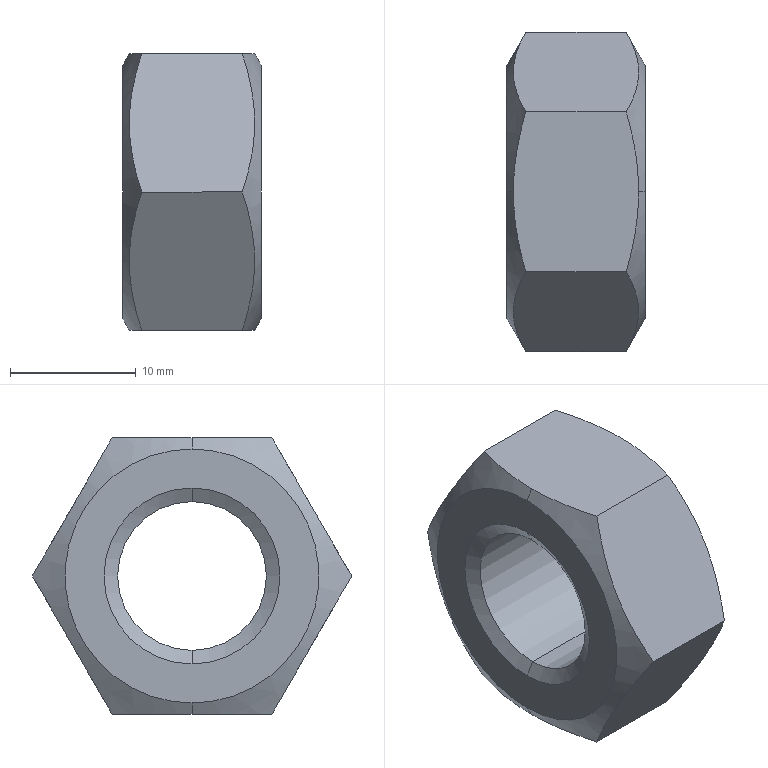Part | STEP file | DIN 934 - M14 x 2 | 1 solid | 18 faces | box 11 x 25.403 x 22 mm | volume 3279 mm3 | cone 8 | plane 8 | cylinder 2 | commonest cylinder face diameters 11.835 x2